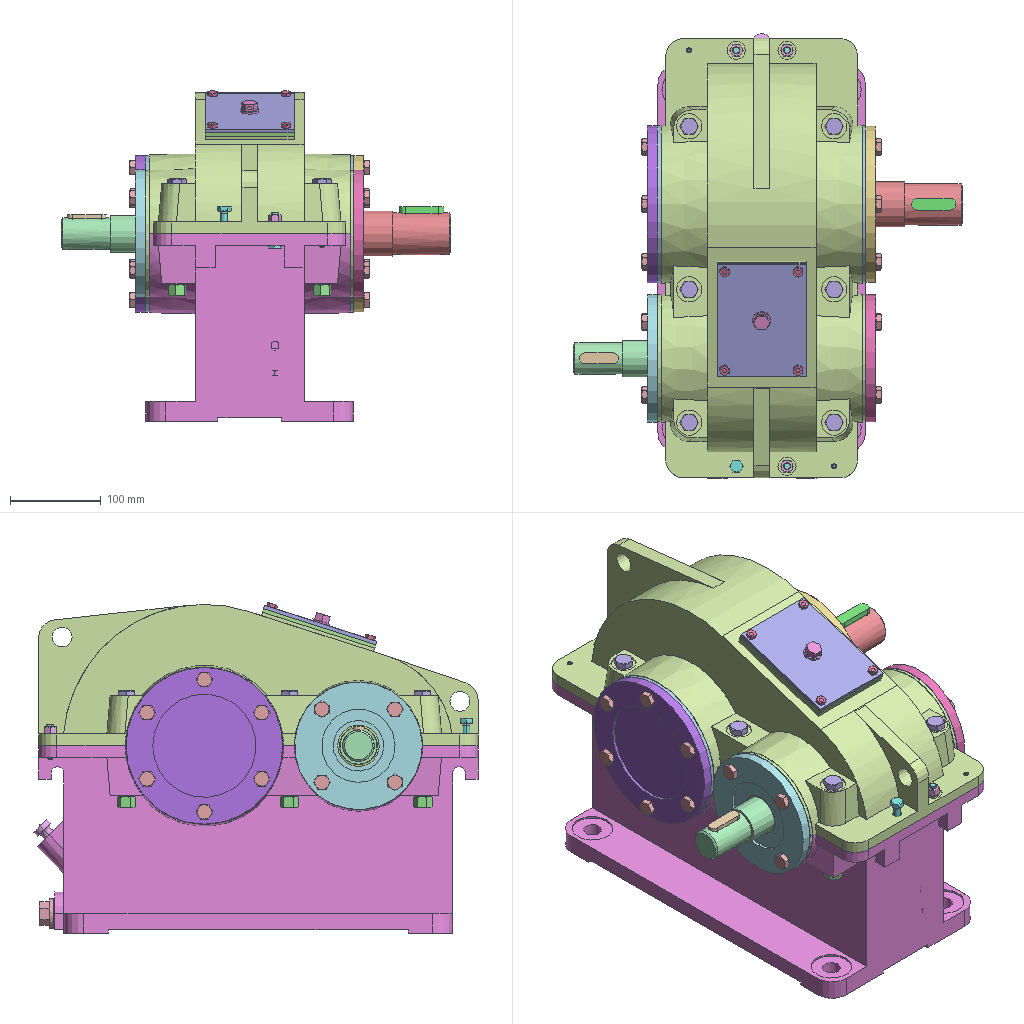Assembly | NX | 37 different items | 90 placed | box 430 x 490 x 365 mm
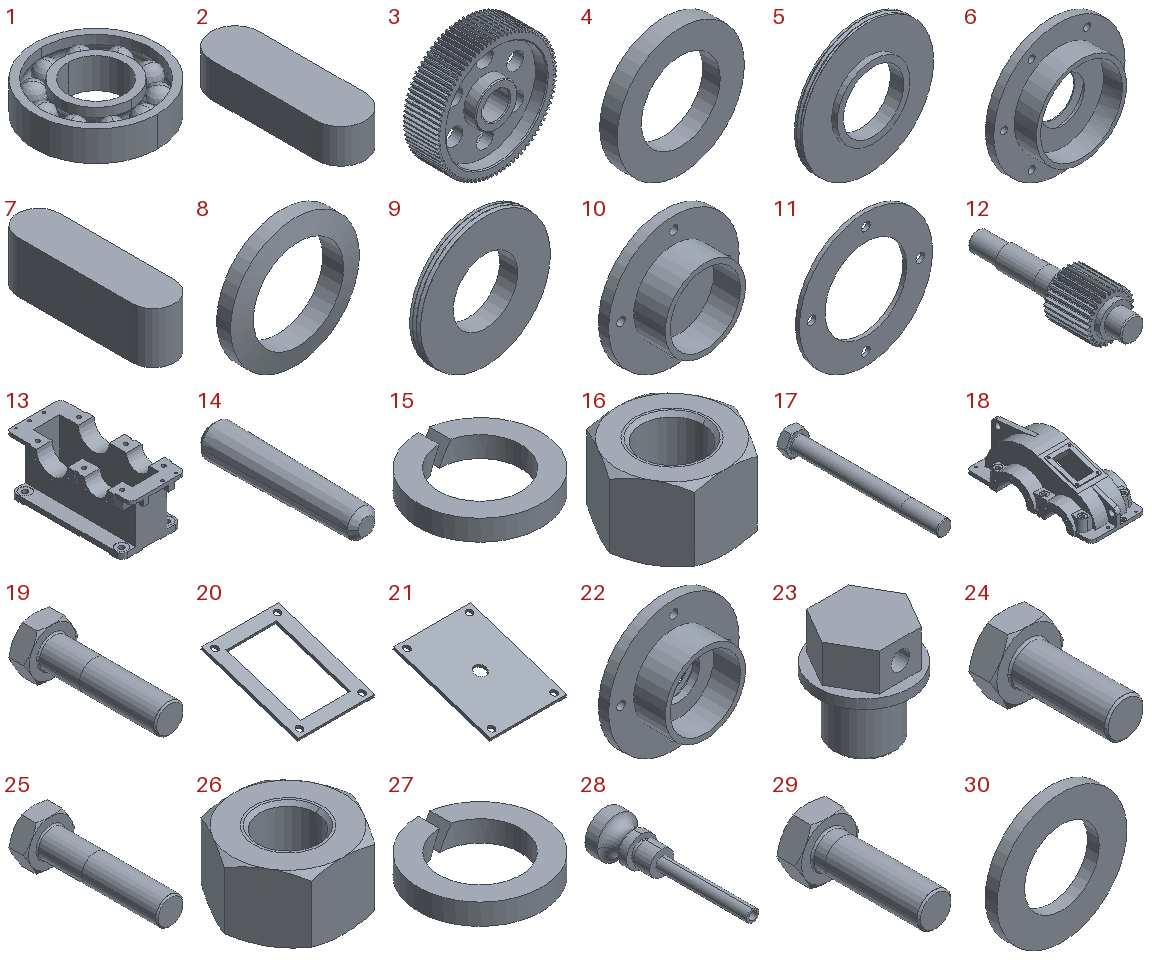Parts list (item | quantity | size | volume | features):
1 | x2 | 110 x 110 x 27 mm | 126080 mm3 | features BREP 12
2 | x1 | 17 x 54 x 12 mm | 10272 mm3 | features DATUM_CSYS 2, BLEND 1, EXTRUDE 1, SKETCH 1
3 | x1 | 270 x 75.43 x 270 mm | 1925103 mm3 | features BREP 88, META 88, DATUM_CSYS 10, EXTRUDE 9, SKETCH 9, EXTRACT_DATUM_AXIS 8, EXTRACT_STRING 8, EXTRACT_DATUM_PLANE 6, Instance Feature 6, EXTRACT_FACE 2, CHAMFER 1, CYLINDER 1, FSET 1, Mirror Feature 1, Pattern Feature 1
4 | x1 | 87 x 12 x 87 mm | 43853 mm3 | features DATUM_CSYS 2, EXTRUDE 1, SKETCH 1
5 | x2 | 117.468 x 12 x 117.468 mm | 63462 mm3 | features DATUM_CSYS 5, SKETCH 4, EXTRUDE 3, SWP104 1
6 | x1 | 173 x 40 x 173 mm | 270737 mm3 | features DATUM_CSYS 10, HOLE PACKAGE 10, SIMPLE HOLE 10, SKETCH 9, EXTRACT_DATUM_AXIS 6, EXTRACT_FACE 6, Instance Feature 5, EXTRUDE 2, DELETE FACE 1, OFFSET_REGION 1, Pattern Feature 1, SWP104 1
7 | x1 | 13 x 49 x 16 mm | 9612 mm3 | features DATUM_CSYS 2, BLEND 1, EXTRUDE 1, OFFSET_REGION 1, SKETCH 1
8 | x1 | 74 x 12 x 74 mm | 21518 mm3 | features DATUM_CSYS 2, SKETCH 1, SWP104 1
9 | x2 | 87 x 12 x 87 mm | 33080 mm3 | features DATUM_CSYS 5, SKETCH 4, EXTRUDE 3, SWP104 1
10 | x1 | 141 x 45 x 141 mm | 224063 mm3 | features DATUM_CSYS 7, HOLE PACKAGE 7, SIMPLE HOLE 7, SKETCH 6, EXTRACT_DATUM_AXIS 4, EXTRACT_FACE 4, Instance Feature 3, EXTRUDE 2, DELETE FACE 1, Pattern Feature 1
11 | x2 | 140 x 4 x 140 mm | 37322 mm3 | features EXTRACT_DATUM_AXIS 8, DATUM_CSYS 6, SKETCH 5, DELETE FACE 4, EXTRACT_DATUM_PLANE 4, EXTRACT_STRING 4, EXTRUDE 4, Instance Feature 3, OFFSET_REGION 3, BREP 1, HOLE PACKAGE 1, Pattern Feature 1, SIMPLE HOLE 1, TRIM BODY 1
12 | x1 | 86.819 x 289 x 86.952 mm | 701275 mm3 | features BREP 27, META 27, DATUM_CSYS 8, EXTRUDE 7, SKETCH 7, EXTRACT_DATUM_AXIS 4, EXTRACT_DATUM_PLANE 2, EXTRACT_STRING 2, BLEND 1, CHAMFER 1, CYLINDER 1, FSET 1, Instance Feature 1, Mirror Feature 1
13 | x1 | 229 x 486.698 x 207 mm | 5319663 mm3 | features DATUM_CSYS 44, SKETCH 43, EXTRUDE 42, EXTRACT_DATUM_AXIS 38, EXTRACT_FACE 32, SIMPLE HOLE 25, EXTRACT_DATUM_PLANE 14, Instance Feature 13, HOLE PACKAGE 10, DRAFT 9, EXTRACT_STRING 8, FSET 6, Mirror Feature 5, BLEND 4, OFFSET_REGION 4, Pattern Feature 2
14 | x2 | 5.848 x 28 x 5.848 mm | 637.188 mm3 | features BREP 1
15 | x6 | 18.4 x 18.4 x 3.1 mm | 446.968 mm3 | features BREP 1
16 | x6 | 20.785 x 18 x 12.2 mm | 3340 mm3 | features BREP 2
17 | x6 | 20.785 x 127.5 x 18 mm | 16910 mm3 | features BREP 2
18 | x1 | 222 x 485 x 156 mm | 3762838 mm3 | features DATUM_CSYS 43, EXTRUDE 42, SKETCH 42, EXTRACT_DATUM_AXIS 38, EXTRACT_FACE 32, SIMPLE HOLE 23, EXTRACT_DATUM_PLANE 14, Instance Feature 13, DRAFT 9, EXTRACT_STRING 8, HOLE PACKAGE 8, FSET 6, Mirror Feature 5, BLEND 4, OFFSET_REGION 4, Pattern Feature 2
19 | x20 | 18.475 x 46.4 x 16 mm | 5287 mm3 | features BREP 2
20 | x1 | 98 x 124.993 x 43.573 mm | 24156 mm3 | features DATUM_CSYS 42, EXTRUDE 41, SKETCH 41, EXTRACT_DATUM_AXIS 38, EXTRACT_FACE 32, SIMPLE HOLE 20, EXTRACT_DATUM_PLANE 14, Instance Feature 13, DRAFT 9, EXTRACT_STRING 8, HOLE PACKAGE 7, FSET 6, Mirror Feature 5, BLEND 4, OFFSET_REGION 4, Pattern Feature 2, TRIM BODY 1
21 | x1 | 98 x 124.993 x 43.573 mm | 49449 mm3 | features DATUM_CSYS 43, EXTRUDE 42, SKETCH 42, EXTRACT_DATUM_AXIS 38, EXTRACT_FACE 32, SIMPLE HOLE 20, EXTRACT_DATUM_PLANE 14, Instance Feature 13, DRAFT 9, EXTRACT_STRING 8, HOLE PACKAGE 7, FSET 6, Mirror Feature 5, BLEND 4, OFFSET_REGION 4, Pattern Feature 2, REPLACE_FACE 1, TRIM BODY 1
22 | x1 | 141 x 45 x 141 mm | 198778 mm3 | features DATUM_CSYS 8, HOLE PACKAGE 7, SIMPLE HOLE 7, SKETCH 7, EXTRACT_DATUM_AXIS 4, EXTRACT_FACE 4, Instance Feature 3, EXTRUDE 2, Pattern Feature 1, SWP104 1
23 | x1 | 20 x 20 x 22 mm | 3665 mm3 | features DATUM_CSYS 6, EXTRUDE 5, SKETCH 5, CHAMFER 1
24 | x4 | 11.547 x 19 x 10 mm | 976.022 mm3 | features BREP 2
25 | x4 | 15.011 x 40.3 x 13 mm | 2917 mm3 | features BREP 2
26 | x4 | 15.011 x 13 x 7.9 mm | 1139 mm3 | features BREP 2
27 | x4 | 12.3 x 12.3 x 2.1 mm | 136.667 mm3 | features BREP 1
28 | x1 | 20 x 74.367 x 20 mm | 5186 mm3 | features BREP 1
29 | x1 | 15.011 x 30.3 x 13 mm | 2414 mm3 | features BREP 2
30 | x1 | 33 x 3 x 33 mm | 1715 mm3 | features DATUM_CSYS 2, EXTRUDE 1, SKETCH 1
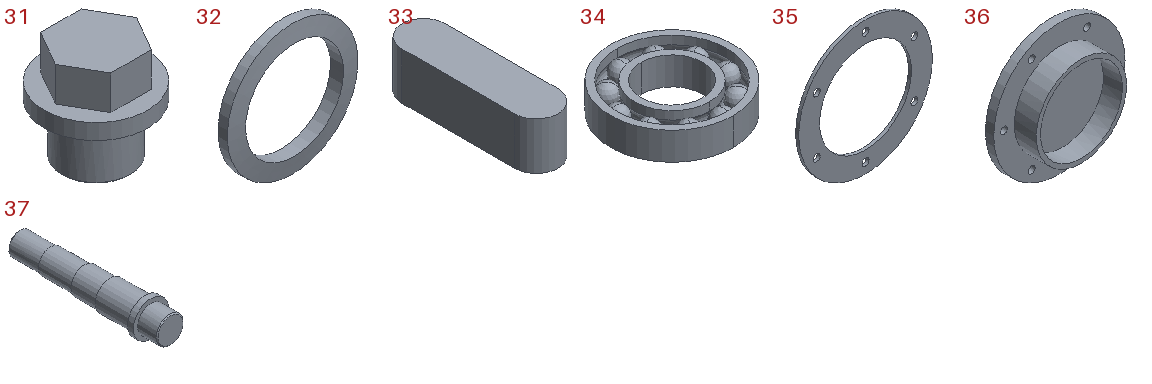31 | x1 | 33 x 33 x 32 mm | 14890 mm3 | features DATUM_CSYS 5, EXTRUDE 4, SKETCH 4, CHAMFER 1
32 | x1 | 56 x 5.63 x 56 mm | 5147 mm3 | features DATUM_CSYS 2, SKETCH 1, SWP104 1
33 | x1 | 12 x 43 x 13 mm | 6306 mm3 | features DATUM_CSYS 2, BLEND 1, EXTRUDE 1, OFFSET_REGION 1, SKETCH 1
34 | x2 | 80 x 80 x 18 mm | 40475 mm3 | features BREP 12
35 | x2 | 173 x 4 x 173 mm | 48010 mm3 | features DATUM_CSYS 2, EXTRUDE 1, SKETCH 1
36 | x1 | 173 x 40 x 173 mm | 317265 mm3 | features DATUM_CSYS 9, HOLE PACKAGE 9, SIMPLE HOLE 9, SKETCH 8, EXTRACT_DATUM_AXIS 6, EXTRACT_FACE 6, Instance Feature 5, EXTRUDE 2, DELETE FACE 1, OFFSET_REGION 1, Pattern Feature 1
37 | x1 | 72 x 309 x 72 mm | 701364 mm3 | features DATUM_CSYS 9, EXTRUDE 8, SKETCH 8, BLEND 2, CHAMFER 1
Mates (type | each side: item.copy, entity, surface, feature):
Fix | 13.1 component
Touch | 18.1 face cylinder Ø87 Hole(27) | 13.1 face cylinder Ø87 Hole(27)
Touch | 18.1 face cylinder Ø119 Hole(28) | 13.1 face cylinder Ø119 Hole(28)
Touch | 18.1 face plane Extrude(2) | 13.1 face plane Extrude(2)
Touch | 11.1 face cylinder Ø90 Hole(7) | 13.1 face cylinder Ø87 Hole(27) | 2 times
Touch | 11.1 face cylinder Pattern Feature [Circular] (12) / Instance[3][0] | 13.1 face cylinder Mirror Feature(45)
Touch | 11.1 face plane Body(1) | 13.1 face plane Mirror Feature(5)
Touch | 11.1 face cylinder Pattern Feature [Circular] (12) / Instance[1][0] | 13.1 face cylinder Pattern Feature [Circular] (43) / Instance[2][0]
Touch | 11.1 face plane Body(1) | 13.1 face plane Extrude(2)
Touch | 22.1 face cylinder Ø46 Hole(3) | 13.1 face cylinder Ø87 Hole(27)
Touch | 22.1 face cylinder Pattern Feature [Circular] (8) / Instance[1][0] | 11.1 face cylinder Pattern Feature [Circular] (12) / Instance[3][0]
Touch | 22.1 face plane Extrude(1) | 11.1 face plane Body(1)
Touch | 34.1 face cylinder Body(1) | 13.1 face cylinder Ø87 Hole(27)
Touch | 34.1 face plane Body(1) | 22.1 face plane Extrude(2)
Touch | 9.1 face cylinder Extrude(4) | 34.1 face surfaceofrevolution Body(2)
Touch | 9.1 face plane Extrude(1) | 34.1 face plane Body(2)
Touch | 12.1 face cylinder Extrude(60) | 13.1 face cylinder Ø87 Hole(27)
Touch | 12.1 face plane Mirror Feature(59) | 9.1 face plane Extrude(2)
Parallel | 12.1 face plane Extrude(62) | 13.1 face plane Extrude(26)
Touch | 9.1 face cylinder Extrude(4) | 12.1 face cylinder Extrude(58)
Touch | 9.1 face plane Extrude(2) | 12.1 face plane Extrude(57)
Touch | 34.1 face cylinder Body(1) | 11.1 face cylinder Ø90 Hole(7)
Touch | 34.1 face plane Body(2) | 9.1 face plane Extrude(1)
Touch | 10.1 face cylinder Ø76 Hole(4) | 11.1 face cylinder Ø90 Hole(7)
Touch | 10.1 face cylinder Pattern Feature [Circular] (8) / Instance[1][0] | 11.1 face cylinder Pattern Feature [Circular] (12) / Instance[2][0]
Touch | 10.1 face plane Extrude(1) | 11.1 face plane Body(1)
Touch | 35.1 face cylinder Extrude(1) | 13.1 face cylinder Ø119 Hole(28)
Touch | 35.1 face cylinder Extrude(1) | 13.1 face cylinder Mirror Feature(45)
Touch | 35.1 face plane Extrude(1) | 13.1 face plane Mirror Feature(5)
Touch | 36.1 face cylinder Extrude(2) | 13.1 face cylinder Ø119 Hole(28)
Touch | 36.1 face cylinder Ø9 Hole(7) | 13.1 face cylinder Mirror Feature(45)
Touch | 36.1 face plane Extrude(1) | 35.1 face plane Extrude(1)
Touch | 1.1 face cylinder Body(1) | 13.1 face cylinder Ø119 Hole(28)
Touch | 1.1 face plane Body(2) | 36.1 face plane Extrude(2)
Touch | 5.1 face cylinder Extrude(2) | 1.1 face cylinder Body(1)
Touch | 5.1 face plane Extrude(2) | 1.1 face plane Body(2)
Touch | 37.1 face cylinder Extrude(4) | 5.1 face cylinder Extrude(4)
Touch | 37.1 face plane Extrude(2) | 5.1 face plane Extrude(1)
Parallel | 13.1 face plane Extrude(26) | 37.1 face plane Extrude(7)
Touch | 2.1 face cylinder Edge Blend(2) | 37.1 face cylinder Edge Blend(8) | 2 times
Touch | 2.1 face plane Extrude(1) | 37.1 face plane Extrude(7)
Touch | 33.1 face cylinder Edge Blend(2) | 12.1 face cylinder Edge Blend(63) | 2 times
Touch | 33.1 face plane Extrude(1) | 12.1 face plane Extrude(62)
Touch | 3.1 face cylinder Extrude(181) | 37.1 face cylinder Extrude(4)
Parallel | 3.1 face plane Extrude(181) | 2.1 face plane Extrude(1)
Distance | 3.1 face plane Cylinder(1) | 37.1 face plane Extrude(2)
Touch | 4.1 face cylinder Extrude(1) | 37.1 face cylinder Extrude(5)
Touch | 4.1 face plane Extrude(1) | 3.1 face plane Cylinder(1)
Touch | 5.1 face cylinder Extrude(4) | 37.1 face cylinder Extrude(4)
Touch | 5.1 face plane Extrude(1) | 4.1 face plane Extrude(1)
Touch | 1.1 face cylinder Body(1) | 37.1 face cylinder Extrude(5)
Touch | 1.1 face plane Body(2) | 5.1 face plane Extrude(2)
Touch | 35.1 face cylinder Extrude(1) | 37.1 face cylinder Extrude(5)
Touch | 35.1 face cylinder Extrude(1) | 13.1 face cylinder Pattern Feature [Circular] (44) / Instance[3][0]
Touch | 35.1 face plane Extrude(1) | 13.1 face plane Extrude(2)
Touch | 6.1 face cylinder Ø114 Hole(5) | 37.1 face cylinder Extrude(6)
Touch | 6.1 face cylinder Pattern Feature [Circular] (7) / Instance[5][0] | 35.1 face cylinder Extrude(1)
Touch | 6.1 face plane Extrude(1) | 35.1 face plane Extrude(1)
Touch | 7.1 face cylinder Edge Blend(2) | 37.1 face cylinder Edge Blend(10) | 2 times
Touch | 7.1 face plane Extrude(1) | 37.1 face plane Extrude(9)
Touch | 20.1 face plane Extrude(22) | 18.1 face plane Extrude(22) | 2 times
Touch | 20.1 face plane Trim Body(48) | 18.1 face plane Extrude(22)
Touch | 21.1 face plane Extrude(22) | 20.1 face plane Extrude(22) | 2 times
Touch | 21.1 face plane Trim Body(48) | 20.1 face plane Extrude(22)
Touch | 24.1 face cylinder Body(1) | 21.1 face cylinder Extrude(22)
Touch | 24.1 face plane Body(1) | 21.1 face plane Extrude(22)
Bond | 21.1 component | assembly component | 2 times
Bond | 24.1 component | assembly component | 4 times
Linear2dPattern | assembly axis | assembly axis | assembly csys | assembly csys | assembly csys | assembly csys
Touch | 23.1 face cylinder Extrude(4) | 21.1 face cylinder Extrude(50)
Touch | 23.1 face plane Extrude(2) | 21.1 face plane Extrude(22)
Touch | 28.1 face cylinder Body(1) | 13.1 face cylinder Ø10 Hole(36)
Touch | 28.1 face plane Body(1) | 13.1 face plane Ø19 Hole(50)
Touch | 30.1 face cylinder Extrude(1) | 13.1 face cylinder Edge Blend(30)
Touch | 30.1 face plane Extrude(1) | 13.1 face plane Ø34 Hole(49)
Touch | 31.1 face cylinder Extrude(2) | 30.1 face cylinder Extrude(1)
Touch | 31.1 face plane Extrude(2) | 30.1 face plane Extrude(1)
Touch | 17.1 face cylinder Body(1) | 18.1 face cylinder Extrude(23)
Touch | 17.1 face plane Body(1) | 18.1 face plane Ø28 Hole(24)
Touch | 15.1 face cylinder Body(1) | 17.1 face cylinder Body(1)
Touch | 15.1 face plane Body(1) | 13.1 face plane Ø28 Hole(25)
Touch | 16.1 face cylinder Body(1) | 17.1 face cylinder Body(1)
Touch | 16.1 face plane Body(1) | 15.1 face plane Body(1)
Fix | assembly component | 9 times
Bond | 16.1 component | assembly component | 10 times
Bond | 17.1 component | assembly component | 10 times
Bond | 15.1 component | assembly component | 10 times
LinearPattern | assembly axis | assembly csys | assembly csys | 24 times
Touch | 32.1 face cylinder Revolve(1) | 12.1 face cylinder Extrude(60)
Touch | 8.1 face cylinder Revolve(1) | 37.1 face cylinder Extrude(6)
Touch | 29.1 face cylinder Body(1) | 18.1 face cylinder Extrude(37)
Touch | 29.1 face plane Body(1) | 13.1 face plane Extrude(37)
Touch | 25.1 face cylinder Body(1) | 18.1 face cylinder Extrude(37)
Touch | 25.1 face plane Body(1) | 13.1 face plane Ø20 Hole(51)
Touch | 27.1 face cylinder Body(1) | 25.1 face cylinder Body(1)
Touch | 27.1 face plane Body(1) | 18.1 face plane Ø20 Hole(49)
Touch | 26.1 face cylinder Body(1) | 25.1 face cylinder Body(1)
Touch | 26.1 face plane Body(1) | 27.1 face plane Body(1)
Bond | 25.1 component | assembly component | 6 times
Bond | 26.1 component | assembly component | 6 times
Bond | 27.1 component | assembly component | 6 times
Bond | 18.1 component | assembly component
Touch | 14.1 face cone Body(1) | 18.1 face cylinder Extrude(37) | 2 times
Touch | 14.1 face plane Body(1) | 18.1 face plane Extrude(1) | 2 times
Touch | 19.1 face cylinder Body(1) | 10.1 face cylinder Ø9 Hole(7)
Touch | 19.1 face plane Body(1) | 10.1 face plane Extrude(1)
Touch | 19.1 face cylinder Body(1) | 6.1 face cylinder Pattern Feature [Circular] (7) / Instance[5][0]
Touch | 19.1 face plane Body(1) | 6.1 face plane Extrude(1)
Touch | 19.1 face cylinder Body(1) | 36.1 face cylinder Ø9 Hole(7)
Touch | 19.1 face plane Body(1) | 36.1 face plane Extrude(1)
Touch | 19.1 face cylinder Body(1) | 22.1 face cylinder Ø9 Hole(7)
Touch | 19.1 face plane Body(1) | 22.1 face plane Extrude(1)
Bond | 19.1 component | assembly component | 20 times
CircularPattern | assembly axis | assembly csys | assembly csys | assembly csys | assembly csys | 2 times
CircularPattern | assembly axis | assembly csys | assembly csys | assembly csys | assembly csys | assembly csys | assembly csys | 2 times